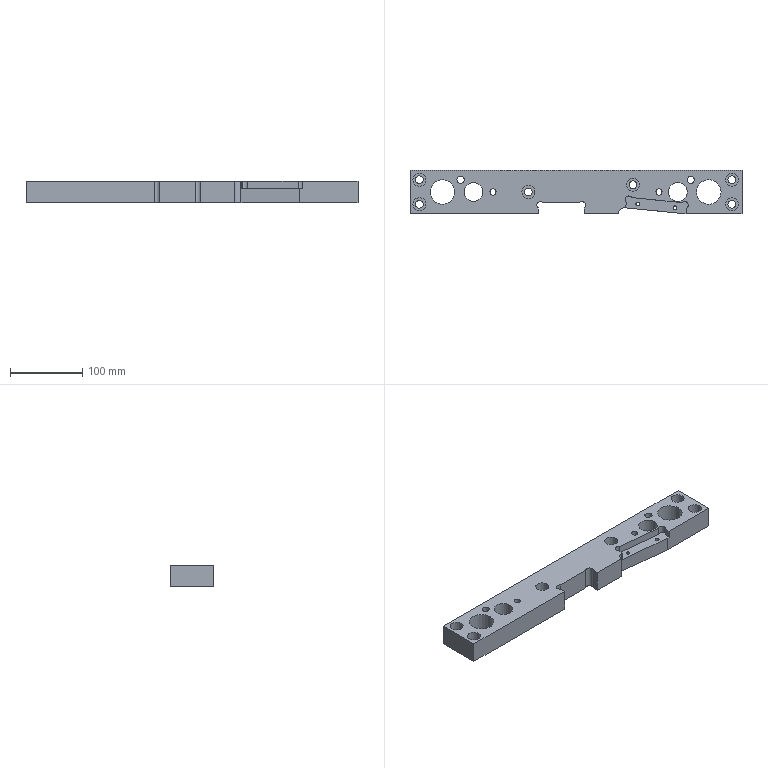Part | NX | features LIN_SOLID_COLOR 2 | 1 solid | 54 faces | box 460 x 60 x 30 mm | volume 644564 mm3 | cylinder 29 | plane 25 | commonest cylinder face diameters 11 x6 18 x6 10 x4 5.2 x2 8.5 x2 10.001 x2
STEP:
#1=CARTESIAN_POINT('',(722.839,118.195,-12.));
#2=VERTEX_POINT('',#1);
#3=CARTESIAN_POINT('',(720.239,118.195,-12.));
#4=DIRECTION('',(0.,0.,-1.));
#5=DIRECTION('',(1.,0.,0.));
#6=AXIS2_PLACEMENT_3D('',#3,#4,#5);
#7=CIRCLE('',#6,2.6);
#8=EDGE_CURVE('',#2,#2,#7,.T.);
#9=ORIENTED_EDGE('',*,*,#8,.T.);
#10=EDGE_LOOP('',(#9));
#11=FACE_BOUND('',#10,.T.);
#12=CARTESIAN_POINT('',(651.88,118.043,-12.));
#13=VERTEX_POINT('',#12);
#14=CARTESIAN_POINT('',(652.678,125.965,-12.));
#15=VERTEX_POINT('',#14);
#16=CARTESIAN_POINT('',(652.581,125.008,-12.));
#17=DIRECTION('',(0.1002,0.995,0.));
#18=VECTOR('',#17,1000.);
#19=LINE('',#16,#18);
#20=EDGE_CURVE('',#13,#15,#19,.T.);
#21=ORIENTED_EDGE('',*,*,#20,.F.);
#22=CARTESIAN_POINT('',(731.751,110.,-12.));
#23=VERTEX_POINT('',#22);
#24=CARTESIAN_POINT('',(646.905,118.544,-12.));
#25=DIRECTION('',(0.995,-0.1002,0.));
#26=VECTOR('',#25,1000.);
#27=LINE('',#24,#26);
#28=EDGE_CURVE('',#13,#23,#27,.T.);
#29=ORIENTED_EDGE('',*,*,#28,.T.);
#30=CARTESIAN_POINT('',(735.495,110.,-12.));
#31=VERTEX_POINT('',#30);
#32=CARTESIAN_POINT('',(667.,110.,-12.));
#33=DIRECTION('',(-1.,0.,0.));
#34=VECTOR('',#33,1000.);
#35=LINE('',#32,#34);
#36=EDGE_CURVE('',#31,#23,#35,.T.);
#37=ORIENTED_EDGE('',*,*,#36,.F.);
#38=CARTESIAN_POINT('',(736.255,117.548,-12.));
#39=VERTEX_POINT('',#38);
#40=CARTESIAN_POINT('',(736.159,116.592,-12.));
#41=DIRECTION('',(0.1002,0.995,0.));
#42=VECTOR('',#41,1000.);
#43=LINE('',#40,#42);
#44=EDGE_CURVE('',#31,#39,#43,.T.);
#45=ORIENTED_EDGE('',*,*,#44,.T.);
#46=CARTESIAN_POINT('',(729.957,125.257,-12.));
#47=VERTEX_POINT('',#46);
#48=CARTESIAN_POINT('',(733.475,121.704,-12.));
#49=DIRECTION('',(0.,0.,1.));
#50=DIRECTION('',(1.,0.,0.));
#51=AXIS2_PLACEMENT_3D('',#48,#49,#50);
#52=CIRCLE('',#51,5.);
#53=EDGE_CURVE('',#39,#47,#52,.T.);
#54=ORIENTED_EDGE('',*,*,#53,.T.);
#55=CARTESIAN_POINT('',(660.386,132.263,-12.));
#56=VERTEX_POINT('',#55);
#57=CARTESIAN_POINT('',(648.408,133.469,-12.));
#58=DIRECTION('',(-0.995,0.1002,0.));
#59=VECTOR('',#58,1000.);
#60=LINE('',#57,#59);
#61=EDGE_CURVE('',#56,#47,#60,.F.);
#62=ORIENTED_EDGE('',*,*,#61,.F.);
#63=CARTESIAN_POINT('',(656.23,129.483,-12.));
#64=DIRECTION('',(0.,0.,1.));
#65=DIRECTION('',(1.,0.,0.));
#66=AXIS2_PLACEMENT_3D('',#63,#64,#65);
#67=CIRCLE('',#66,5.);
#68=EDGE_CURVE('',#56,#15,#67,.T.);
#69=ORIENTED_EDGE('',*,*,#68,.T.);
#70=EDGE_LOOP('',(#21,#29,#37,#45,#54,#62,#69));
#71=FACE_BOUND('',#70,.T.);
#72=CARTESIAN_POINT('',(671.101,123.405,-12.));
#73=VERTEX_POINT('',#72);
#74=CARTESIAN_POINT('',(668.501,123.405,-12.));
#75=DIRECTION('',(0.,0.,-1.));
#76=DIRECTION('',(1.,0.,0.));
#77=AXIS2_PLACEMENT_3D('',#74,#75,#76);
#78=CIRCLE('',#77,2.6);
#79=EDGE_CURVE('',#73,#73,#78,.T.);
#80=ORIENTED_EDGE('',*,*,#79,.T.);
#81=EDGE_LOOP('',(#80));
#82=FACE_BOUND('',#81,.T.);
#83=CARTESIAN_POINT('',(647.606,125.509,-12.));
#84=DIRECTION('',(0.,0.,1.));
#85=DIRECTION('',(-0.9923,0.1236,0.));
#86=AXIS2_PLACEMENT_3D('',#83,#84,#85);
#87=PLANE('',#86);
#88=ADVANCED_FACE('',(#11,#71,#82),#87,.T.);
#89=CARTESIAN_POINT('',(693.75,140.,-1.5));
#90=VERTEX_POINT('',#89);
#91=CARTESIAN_POINT('',(698.,140.,-1.5));
#92=DIRECTION('',(0.,0.,1.));
#93=DIRECTION('',(-1.,0.,0.));
#94=AXIS2_PLACEMENT_3D('',#91,#92,#93);
#95=CIRCLE('',#94,4.25);
#96=EDGE_CURVE('',#90,#90,#95,.T.);
#97=ORIENTED_EDGE('',*,*,#96,.F.);
#98=EDGE_LOOP('',(#97));
#99=FACE_BOUND('',#98,.T.);
#100=CARTESIAN_POINT('',(472.25,140.,-1.5));
#101=VERTEX_POINT('',#100);
#102=CARTESIAN_POINT('',(468.,140.,-1.5));
#103=DIRECTION('',(0.,0.,-1.));
#104=DIRECTION('',(1.,0.,0.));
#105=AXIS2_PLACEMENT_3D('',#102,#103,#104);
#106=CIRCLE('',#105,4.25);
#107=EDGE_CURVE('',#101,#101,#106,.T.);
#108=ORIENTED_EDGE('',*,*,#107,.T.);
#109=EDGE_LOOP('',(#108));
#110=FACE_BOUND('',#109,.T.);
#111=CARTESIAN_POINT('',(671.,150.,-1.5));
#112=VERTEX_POINT('',#111);
#113=CARTESIAN_POINT('',(662.,150.,-1.5));
#114=DIRECTION('',(0.,0.,1.));
#115=DIRECTION('',(1.,0.,0.));
#116=AXIS2_PLACEMENT_3D('',#113,#114,#115);
#117=CIRCLE('',#116,9.);
#118=EDGE_CURVE('',#112,#112,#117,.T.);
#119=ORIENTED_EDGE('',*,*,#118,.F.);
#120=EDGE_LOOP('',(#119));
#121=FACE_BOUND('',#120,.T.);
#122=CARTESIAN_POINT('',(415.,140.,-1.5));
#123=VERTEX_POINT('',#122);
#124=CARTESIAN_POINT('',(398.,140.,-1.5));
#125=DIRECTION('',(0.,0.,1.));
#126=DIRECTION('',(1.,0.,0.));
#127=AXIS2_PLACEMENT_3D('',#124,#125,#126);
#128=CIRCLE('',#127,17.);
#129=EDGE_CURVE('',#123,#123,#128,.F.);
#130=ORIENTED_EDGE('',*,*,#129,.T.);
#131=EDGE_LOOP('',(#130));
#132=FACE_BOUND('',#131,.T.);
#133=CARTESIAN_POINT('',(784.,140.,-1.5));
#134=VERTEX_POINT('',#133);
#135=CARTESIAN_POINT('',(767.,140.,-1.5));
#136=DIRECTION('',(0.,0.,1.));
#137=DIRECTION('',(1.,0.,0.));
#138=AXIS2_PLACEMENT_3D('',#135,#136,#137);
#139=CIRCLE('',#138,17.);
#140=EDGE_CURVE('',#134,#134,#139,.T.);
#141=ORIENTED_EDGE('',*,*,#140,.F.);
#142=EDGE_LOOP('',(#141));
#143=FACE_BOUND('',#142,.T.);
#144=CARTESIAN_POINT('',(375.,157.,-1.5));
#145=VERTEX_POINT('',#144);
#146=CARTESIAN_POINT('',(366.,157.,-1.5));
#147=DIRECTION('',(0.,0.,1.));
#148=DIRECTION('',(1.,0.,0.));
#149=AXIS2_PLACEMENT_3D('',#146,#147,#148);
#150=CIRCLE('',#149,9.);
#151=EDGE_CURVE('',#145,#145,#150,.F.);
#152=ORIENTED_EDGE('',*,*,#151,.T.);
#153=EDGE_LOOP('',(#152));
#154=FACE_BOUND('',#153,.T.);
#155=CARTESIAN_POINT('',(375.,123.,-1.5));
#156=VERTEX_POINT('',#155);
#157=CARTESIAN_POINT('',(366.,123.,-1.5));
#158=DIRECTION('',(0.,0.,1.));
#159=DIRECTION('',(1.,0.,0.));
#160=AXIS2_PLACEMENT_3D('',#157,#158,#159);
#161=CIRCLE('',#160,9.);
#162=EDGE_CURVE('',#156,#156,#161,.F.);
#163=ORIENTED_EDGE('',*,*,#162,.T.);
#164=EDGE_LOOP('',(#163));
#165=FACE_BOUND('',#164,.T.);
#166=CARTESIAN_POINT('',(428.004,157.,-1.5));
#167=VERTEX_POINT('',#166);
#168=CARTESIAN_POINT('',(423.003,157.,-1.5));
#169=DIRECTION('',(0.,0.,1.));
#170=DIRECTION('',(1.,0.,0.));
#171=AXIS2_PLACEMENT_3D('',#168,#169,#170);
#172=CIRCLE('',#171,5.);
#173=EDGE_CURVE('',#167,#167,#172,.F.);
#174=ORIENTED_EDGE('',*,*,#173,.T.);
#175=EDGE_LOOP('',(#174));
#176=FACE_BOUND('',#175,.T.);
#177=CARTESIAN_POINT('',(526.,140.,-1.5));
#178=VERTEX_POINT('',#177);
#179=CARTESIAN_POINT('',(517.,140.,-1.5));
#180=DIRECTION('',(0.,0.,1.));
#181=DIRECTION('',(1.,0.,0.));
#182=AXIS2_PLACEMENT_3D('',#179,#180,#181);
#183=CIRCLE('',#182,9.);
#184=EDGE_CURVE('',#178,#178,#183,.F.);
#185=ORIENTED_EDGE('',*,*,#184,.T.);
#186=EDGE_LOOP('',(#185));
#187=FACE_BOUND('',#186,.T.);
#188=CARTESIAN_POINT('',(746.997,157.,-1.5));
#189=VERTEX_POINT('',#188);
#190=CARTESIAN_POINT('',(741.997,157.,-1.5));
#191=DIRECTION('',(0.,0.,1.));
#192=DIRECTION('',(1.,0.,0.));
#193=AXIS2_PLACEMENT_3D('',#190,#191,#192);
#194=CIRCLE('',#193,5.);
#195=EDGE_CURVE('',#189,#189,#194,.F.);
#196=ORIENTED_EDGE('',*,*,#195,.T.);
#197=EDGE_LOOP('',(#196));
#198=FACE_BOUND('',#197,.T.);
#199=CARTESIAN_POINT('',(808.,157.,-1.5));
#200=VERTEX_POINT('',#199);
#201=CARTESIAN_POINT('',(799.,157.,-1.5));
#202=DIRECTION('',(0.,0.,1.));
#203=DIRECTION('',(1.,0.,0.));
#204=AXIS2_PLACEMENT_3D('',#201,#202,#203);
#205=CIRCLE('',#204,9.);
#206=EDGE_CURVE('',#200,#200,#205,.F.);
#207=ORIENTED_EDGE('',*,*,#206,.T.);
#208=EDGE_LOOP('',(#207));
#209=FACE_BOUND('',#208,.T.);
#210=CARTESIAN_POINT('',(808.,123.,-1.5));
#211=VERTEX_POINT('',#210);
#212=CARTESIAN_POINT('',(799.,123.,-1.5));
#213=DIRECTION('',(0.,0.,1.));
#214=DIRECTION('',(1.,0.,0.));
#215=AXIS2_PLACEMENT_3D('',#212,#213,#214);
#216=CIRCLE('',#215,9.);
#217=EDGE_CURVE('',#211,#211,#216,.F.);
#218=ORIENTED_EDGE('',*,*,#217,.T.);
#219=EDGE_LOOP('',(#218));
#220=FACE_BOUND('',#219,.T.);
#221=CARTESIAN_POINT('',(737.,140.,-1.5));
#222=VERTEX_POINT('',#221);
#223=CARTESIAN_POINT('',(724.,140.,-1.5));
#224=DIRECTION('',(0.,0.,-1.));
#225=DIRECTION('',(1.,0.,0.));
#226=AXIS2_PLACEMENT_3D('',#223,#224,#225);
#227=CIRCLE('',#226,13.);
#228=EDGE_CURVE('',#222,#222,#227,.T.);
#229=ORIENTED_EDGE('',*,*,#228,.T.);
#230=EDGE_LOOP('',(#229));
#231=FACE_BOUND('',#230,.T.);
#232=CARTESIAN_POINT('',(454.,140.,-1.5));
#233=VERTEX_POINT('',#232);
#234=CARTESIAN_POINT('',(441.,140.,-1.5));
#235=DIRECTION('',(0.,0.,-1.));
#236=DIRECTION('',(1.,0.,0.));
#237=AXIS2_PLACEMENT_3D('',#234,#235,#236);
#238=CIRCLE('',#237,13.);
#239=EDGE_CURVE('',#233,#233,#238,.F.);
#240=ORIENTED_EDGE('',*,*,#239,.F.);
#241=EDGE_LOOP('',(#240));
#242=FACE_BOUND('',#241,.T.);
#243=CARTESIAN_POINT('',(530.5,110.,-1.5));
#244=VERTEX_POINT('',#243);
#245=CARTESIAN_POINT('',(530.5,117.961,-1.5));
#246=VERTEX_POINT('',#245);
#247=CARTESIAN_POINT('',(530.5,0.,-1.5));
#248=DIRECTION('',(0.,1.,0.));
#249=VECTOR('',#248,1000.);
#250=LINE('',#247,#249);
#251=EDGE_CURVE('',#244,#246,#250,.T.);
#252=ORIENTED_EDGE('',*,*,#251,.T.);
#253=CARTESIAN_POINT('',(537.539,125.,-1.5));
#254=VERTEX_POINT('',#253);
#255=CARTESIAN_POINT('',(533.682,121.818,-1.5));
#256=DIRECTION('',(0.,0.,-1.));
#257=DIRECTION('',(1.,0.,0.));
#258=AXIS2_PLACEMENT_3D('',#255,#256,#257);
#259=CIRCLE('',#258,5.);
#260=EDGE_CURVE('',#246,#254,#259,.T.);
#261=ORIENTED_EDGE('',*,*,#260,.T.);
#262=CARTESIAN_POINT('',(587.461,125.,-1.5));
#263=VERTEX_POINT('',#262);
#264=CARTESIAN_POINT('',(630.2,125.,-1.5));
#265=DIRECTION('',(-1.,0.,0.));
#266=VECTOR('',#265,1000.);
#267=LINE('',#264,#266);
#268=EDGE_CURVE('',#263,#254,#267,.T.);
#269=ORIENTED_EDGE('',*,*,#268,.F.);
#270=CARTESIAN_POINT('',(594.5,117.961,-1.5));
#271=VERTEX_POINT('',#270);
#272=CARTESIAN_POINT('',(591.318,121.818,-1.5));
#273=DIRECTION('',(0.,0.,-1.));
#274=DIRECTION('',(1.,0.,0.));
#275=AXIS2_PLACEMENT_3D('',#272,#273,#274);
#276=CIRCLE('',#275,5.);
#277=EDGE_CURVE('',#263,#271,#276,.T.);
#278=ORIENTED_EDGE('',*,*,#277,.T.);
#279=CARTESIAN_POINT('',(594.5,110.,-1.5));
#280=VERTEX_POINT('',#279);
#281=CARTESIAN_POINT('',(594.5,173.255,-1.5));
#282=DIRECTION('',(0.,-1.,0.));
#283=VECTOR('',#282,1000.);
#284=LINE('',#281,#283);
#285=EDGE_CURVE('',#271,#280,#284,.T.);
#286=ORIENTED_EDGE('',*,*,#285,.T.);
#287=CARTESIAN_POINT('',(642.024,110.,-1.5));
#288=VERTEX_POINT('',#287);
#289=CARTESIAN_POINT('',(667.,110.,-1.5));
#290=DIRECTION('',(-1.,0.,0.));
#291=VECTOR('',#290,1000.);
#292=LINE('',#289,#291);
#293=EDGE_CURVE('',#280,#288,#292,.F.);
#294=ORIENTED_EDGE('',*,*,#293,.T.);
#295=CARTESIAN_POINT('',(642.124,110.985,-1.5));
#296=VERTEX_POINT('',#295);
#297=CARTESIAN_POINT('',(648.212,171.442,-1.5));
#298=DIRECTION('',(-0.1002,-0.995,0.));
#299=VECTOR('',#298,1000.);
#300=LINE('',#297,#299);
#301=EDGE_CURVE('',#296,#288,#300,.T.);
#302=ORIENTED_EDGE('',*,*,#301,.F.);
#303=CARTESIAN_POINT('',(650.885,118.144,-1.5));
#304=VERTEX_POINT('',#303);
#305=CARTESIAN_POINT('',(650.083,110.184,-1.5));
#306=DIRECTION('',(0.,0.,1.));
#307=DIRECTION('',(1.,0.,0.));
#308=AXIS2_PLACEMENT_3D('',#305,#306,#307);
#309=CIRCLE('',#308,8.);
#310=EDGE_CURVE('',#304,#296,#309,.T.);
#311=ORIENTED_EDGE('',*,*,#310,.F.);
#312=CARTESIAN_POINT('',(651.88,118.043,-1.5));
#313=VERTEX_POINT('',#312);
#314=CARTESIAN_POINT('',(624.913,120.759,-1.5));
#315=DIRECTION('',(0.995,-0.1002,0.));
#316=VECTOR('',#315,1000.);
#317=LINE('',#314,#316);
#318=EDGE_CURVE('',#304,#313,#317,.T.);
#319=ORIENTED_EDGE('',*,*,#318,.T.);
#320=CARTESIAN_POINT('',(652.678,125.965,-1.5));
#321=VERTEX_POINT('',#320);
#322=CARTESIAN_POINT('',(657.167,170.54,-1.5));
#323=DIRECTION('',(0.1002,0.995,0.));
#324=VECTOR('',#323,1000.);
#325=LINE('',#322,#324);
#326=EDGE_CURVE('',#313,#321,#325,.T.);
#327=ORIENTED_EDGE('',*,*,#326,.T.);
#328=CARTESIAN_POINT('',(660.386,132.263,-1.5));
#329=VERTEX_POINT('',#328);
#330=CARTESIAN_POINT('',(656.23,129.483,-1.5));
#331=DIRECTION('',(0.,0.,1.));
#332=DIRECTION('',(1.,0.,0.));
#333=AXIS2_PLACEMENT_3D('',#330,#331,#332);
#334=CIRCLE('',#333,5.);
#335=EDGE_CURVE('',#329,#321,#334,.T.);
#336=ORIENTED_EDGE('',*,*,#335,.F.);
#337=CARTESIAN_POINT('',(729.957,125.257,-1.5));
#338=VERTEX_POINT('',#337);
#339=CARTESIAN_POINT('',(626.416,135.684,-1.5));
#340=DIRECTION('',(-0.995,0.1002,0.));
#341=VECTOR('',#340,1000.);
#342=LINE('',#339,#341);
#343=EDGE_CURVE('',#338,#329,#342,.T.);
#344=ORIENTED_EDGE('',*,*,#343,.F.);
#345=CARTESIAN_POINT('',(736.255,117.548,-1.5));
#346=VERTEX_POINT('',#345);
#347=CARTESIAN_POINT('',(733.475,121.704,-1.5));
#348=DIRECTION('',(0.,0.,1.));
#349=DIRECTION('',(1.,0.,0.));
#350=AXIS2_PLACEMENT_3D('',#347,#348,#349);
#351=CIRCLE('',#350,5.);
#352=EDGE_CURVE('',#346,#338,#351,.T.);
#353=ORIENTED_EDGE('',*,*,#352,.F.);
#354=CARTESIAN_POINT('',(735.495,110.,-1.5));
#355=VERTEX_POINT('',#354);
#356=CARTESIAN_POINT('',(740.744,162.123,-1.5));
#357=DIRECTION('',(-0.1002,-0.995,0.));
#358=VECTOR('',#357,1000.);
#359=LINE('',#356,#358);
#360=EDGE_CURVE('',#346,#355,#359,.T.);
#361=ORIENTED_EDGE('',*,*,#360,.T.);
#362=CARTESIAN_POINT('',(813.,110.,-1.5));
#363=VERTEX_POINT('',#362);
#364=CARTESIAN_POINT('',(667.,110.,-1.5));
#365=DIRECTION('',(-1.,0.,0.));
#366=VECTOR('',#365,1000.);
#367=LINE('',#364,#366);
#368=EDGE_CURVE('',#355,#363,#367,.F.);
#369=ORIENTED_EDGE('',*,*,#368,.T.);
#370=CARTESIAN_POINT('',(813.,170.,-1.5));
#371=VERTEX_POINT('',#370);
#372=CARTESIAN_POINT('',(813.,30.,-1.5));
#373=DIRECTION('',(0.,-1.,0.));
#374=VECTOR('',#373,1000.);
#375=LINE('',#372,#374);
#376=EDGE_CURVE('',#371,#363,#375,.T.);
#377=ORIENTED_EDGE('',*,*,#376,.F.);
#378=CARTESIAN_POINT('',(353.,170.,-1.5));
#379=VERTEX_POINT('',#378);
#380=CARTESIAN_POINT('',(667.,170.,-1.5));
#381=DIRECTION('',(1.,0.,0.));
#382=VECTOR('',#381,1000.);
#383=LINE('',#380,#382);
#384=EDGE_CURVE('',#371,#379,#383,.F.);
#385=ORIENTED_EDGE('',*,*,#384,.T.);
#386=CARTESIAN_POINT('',(353.,110.,-1.5));
#387=VERTEX_POINT('',#386);
#388=CARTESIAN_POINT('',(353.,30.,-1.5));
#389=DIRECTION('',(0.,-1.,0.));
#390=VECTOR('',#389,1000.);
#391=LINE('',#388,#390);
#392=EDGE_CURVE('',#379,#387,#391,.T.);
#393=ORIENTED_EDGE('',*,*,#392,.T.);
#394=CARTESIAN_POINT('',(667.,110.,-1.5));
#395=DIRECTION('',(-1.,0.,0.));
#396=VECTOR('',#395,1000.);
#397=LINE('',#394,#396);
#398=EDGE_CURVE('',#387,#244,#397,.F.);
#399=ORIENTED_EDGE('',*,*,#398,.T.);
#400=EDGE_LOOP('',(#252,#261,#269,#278,#286,#294,#302,#311,#319,#327,#336,#344,#353,#361,#369,#377,#385,#393,#399));
#401=FACE_BOUND('',#400,.T.);
#402=CARTESIAN_POINT('',(630.2,173.255,-1.5));
#403=DIRECTION('',(0.,0.,1.));
#404=DIRECTION('',(1.,0.,0.));
#405=AXIS2_PLACEMENT_3D('',#402,#403,#404);
#406=PLANE('',#405);
#407=ADVANCED_FACE('',(#99,#110,#121,#132,#143,#154,#165,#176,#187,#198,#209,#220,#231,#242,#401),#406,.T.);
#408=CARTESIAN_POINT('',(665.901,123.405,-31.5));
#409=VERTEX_POINT('',#408);
#410=CARTESIAN_POINT('',(668.501,123.405,-31.5));
#411=DIRECTION('',(0.,0.,-1.));
#412=DIRECTION('',(-1.,0.,0.));
#413=AXIS2_PLACEMENT_3D('',#410,#411,#412);
#414=CIRCLE('',#413,2.6);
#415=EDGE_CURVE('',#409,#409,#414,.T.);
#416=ORIENTED_EDGE('',*,*,#415,.F.);
#417=EDGE_LOOP('',(#416));
#418=FACE_BOUND('',#417,.T.);
#419=CARTESIAN_POINT('',(717.639,118.195,-31.5));
#420=VERTEX_POINT('',#419);
#421=CARTESIAN_POINT('',(720.239,118.195,-31.5));
#422=DIRECTION('',(0.,0.,-1.));
#423=DIRECTION('',(-1.,0.,0.));
#424=AXIS2_PLACEMENT_3D('',#421,#422,#423);
#425=CIRCLE('',#424,2.6);
#426=EDGE_CURVE('',#420,#420,#425,.T.);
#427=ORIENTED_EDGE('',*,*,#426,.F.);
#428=EDGE_LOOP('',(#427));
#429=FACE_BOUND('',#428,.T.);
#430=CARTESIAN_POINT('',(463.75,140.,-31.5));
#431=VERTEX_POINT('',#430);
#432=CARTESIAN_POINT('',(468.,140.,-31.5));
#433=DIRECTION('',(0.,0.,-1.));
#434=DIRECTION('',(-1.,0.,0.));
#435=AXIS2_PLACEMENT_3D('',#432,#433,#434);
#436=CIRCLE('',#435,4.25);
#437=EDGE_CURVE('',#431,#431,#436,.T.);
#438=ORIENTED_EDGE('',*,*,#437,.F.);
#439=EDGE_LOOP('',(#438));
#440=FACE_BOUND('',#439,.T.);
#441=CARTESIAN_POINT('',(693.75,140.,-31.5));
#442=VERTEX_POINT('',#441);
#443=CARTESIAN_POINT('',(698.,140.,-31.5));
#444=DIRECTION('',(0.,0.,-1.));
#445=DIRECTION('',(-1.,0.,0.));
#446=AXIS2_PLACEMENT_3D('',#443,#444,#445);
#447=CIRCLE('',#446,4.25);
#448=EDGE_CURVE('',#442,#442,#447,.T.);
#449=ORIENTED_EDGE('',*,*,#448,.F.);
#450=EDGE_LOOP('',(#449));
#451=FACE_BOUND('',#450,.T.);
#452=CARTESIAN_POINT('',(428.,140.,-31.5));
#453=VERTEX_POINT('',#452);
#454=CARTESIAN_POINT('',(441.,140.,-31.5));
#455=DIRECTION('',(0.,0.,1.));
#456=DIRECTION('',(-1.,0.,0.));
#457=AXIS2_PLACEMENT_3D('',#454,#455,#456);
#458=CIRCLE('',#457,13.);
#459=EDGE_CURVE('',#453,#453,#458,.F.);
#460=ORIENTED_EDGE('',*,*,#459,.F.);
#461=EDGE_LOOP('',(#460));
#462=FACE_BOUND('',#461,.T.);
#463=CARTESIAN_POINT('',(711.,140.,-31.5));
#464=VERTEX_POINT('',#463);
#465=CARTESIAN_POINT('',(724.,140.,-31.5));
#466=DIRECTION('',(0.,0.,1.));
#467=DIRECTION('',(-1.,0.,0.));
#468=AXIS2_PLACEMENT_3D('',#465,#466,#467);
#469=CIRCLE('',#468,13.);
#470=EDGE_CURVE('',#464,#464,#469,.T.);
#471=ORIENTED_EDGE('',*,*,#470,.T.);
#472=EDGE_LOOP('',(#471));
#473=FACE_BOUND('',#472,.T.);
#474=CARTESIAN_POINT('',(793.5,123.,-31.5));
#475=VERTEX_POINT('',#474);
#476=CARTESIAN_POINT('',(799.,123.,-31.5));
#477=DIRECTION('',(0.,0.,-1.));
#478=DIRECTION('',(-1.,0.,0.));
#479=AXIS2_PLACEMENT_3D('',#476,#477,#478);
#480=CIRCLE('',#479,5.5);
#481=EDGE_CURVE('',#475,#475,#480,.F.);
#482=ORIENTED_EDGE('',*,*,#481,.T.);
#483=EDGE_LOOP('',(#482));
#484=FACE_BOUND('',#483,.T.);
#485=CARTESIAN_POINT('',(793.5,157.,-31.5));
#486=VERTEX_POINT('',#485);
#487=CARTESIAN_POINT('',(799.,157.,-31.5));
#488=DIRECTION('',(0.,0.,-1.));
#489=DIRECTION('',(-1.,0.,0.));
#490=AXIS2_PLACEMENT_3D('',#487,#488,#489);
#491=CIRCLE('',#490,5.5);
#492=EDGE_CURVE('',#486,#486,#491,.F.);
#493=ORIENTED_EDGE('',*,*,#492,.T.);
#494=EDGE_LOOP('',(#493));
#495=FACE_BOUND('',#494,.T.);
#496=CARTESIAN_POINT('',(736.996,157.,-31.5));
#497=VERTEX_POINT('',#496);
#498=CARTESIAN_POINT('',(741.997,157.,-31.5));
#499=DIRECTION('',(0.,0.,-1.));
#500=DIRECTION('',(-1.,0.,0.));
#501=AXIS2_PLACEMENT_3D('',#498,#499,#500);
#502=CIRCLE('',#501,5.);
#503=EDGE_CURVE('',#497,#497,#502,.F.);
#504=ORIENTED_EDGE('',*,*,#503,.T.);
#505=EDGE_LOOP('',(#504));
#506=FACE_BOUND('',#505,.T.);
#507=CARTESIAN_POINT('',(511.5,140.,-31.5));
#508=VERTEX_POINT('',#507);
#509=CARTESIAN_POINT('',(517.,140.,-31.5));
#510=DIRECTION('',(0.,0.,-1.));
#511=DIRECTION('',(-1.,0.,0.));
#512=AXIS2_PLACEMENT_3D('',#509,#510,#511);
#513=CIRCLE('',#512,5.5);
#514=EDGE_CURVE('',#508,#508,#513,.F.);
#515=ORIENTED_EDGE('',*,*,#514,.T.);
#516=EDGE_LOOP('',(#515));
#517=FACE_BOUND('',#516,.T.);
#518=CARTESIAN_POINT('',(379.,140.,-31.5));
#519=VERTEX_POINT('',#518);
#520=CARTESIAN_POINT('',(398.,140.,-31.5));
#521=DIRECTION('',(0.,0.,-1.));
#522=DIRECTION('',(-1.,0.,0.));
#523=AXIS2_PLACEMENT_3D('',#520,#521,#522);
#524=CIRCLE('',#523,19.);
#525=EDGE_CURVE('',#519,#519,#524,.T.);
#526=ORIENTED_EDGE('',*,*,#525,.F.);
#527=EDGE_LOOP('',(#526));
#528=FACE_BOUND('',#527,.T.);
#529=CARTESIAN_POINT('',(748.,140.,-31.5));
#530=VERTEX_POINT('',#529);
#531=CARTESIAN_POINT('',(767.,140.,-31.5));
#532=DIRECTION('',(0.,0.,-1.));
#533=DIRECTION('',(-1.,0.,0.));
#534=AXIS2_PLACEMENT_3D('',#531,#532,#533);
#535=CIRCLE('',#534,19.);
#536=EDGE_CURVE('',#530,#530,#535,.F.);
#537=ORIENTED_EDGE('',*,*,#536,.T.);
#538=EDGE_LOOP('',(#537));
#539=FACE_BOUND('',#538,.T.);
#540=CARTESIAN_POINT('',(360.5,157.,-31.5));
#541=VERTEX_POINT('',#540);
#542=CARTESIAN_POINT('',(366.,157.,-31.5));
#543=DIRECTION('',(0.,0.,-1.));
#544=DIRECTION('',(-1.,0.,0.));
#545=AXIS2_PLACEMENT_3D('',#542,#543,#544);
#546=CIRCLE('',#545,5.5);
#547=EDGE_CURVE('',#541,#541,#546,.F.);
#548=ORIENTED_EDGE('',*,*,#547,.T.);
#549=EDGE_LOOP('',(#548));
#550=FACE_BOUND('',#549,.T.);
#551=CARTESIAN_POINT('',(360.5,123.,-31.5));
#552=VERTEX_POINT('',#551);
#553=CARTESIAN_POINT('',(366.,123.,-31.5));
#554=DIRECTION('',(0.,0.,-1.));
#555=DIRECTION('',(-1.,0.,0.));
#556=AXIS2_PLACEMENT_3D('',#553,#554,#555);
#557=CIRCLE('',#556,5.5);
#558=EDGE_CURVE('',#552,#552,#557,.F.);
#559=ORIENTED_EDGE('',*,*,#558,.T.);
#560=EDGE_LOOP('',(#559));
#561=FACE_BOUND('',#560,.T.);
#562=CARTESIAN_POINT('',(418.003,157.,-31.5));
#563=VERTEX_POINT('',#562);
#564=CARTESIAN_POINT('',(423.003,157.,-31.5));
#565=DIRECTION('',(0.,0.,-1.));
#566=DIRECTION('',(-1.,0.,0.));
#567=AXIS2_PLACEMENT_3D('',#564,#565,#566);
#568=CIRCLE('',#567,5.);
#569=EDGE_CURVE('',#563,#563,#568,.T.);
#570=ORIENTED_EDGE('',*,*,#569,.F.);
#571=EDGE_LOOP('',(#570));
#572=FACE_BOUND('',#571,.T.);
#573=CARTESIAN_POINT('',(656.5,150.,-31.5));
#574=VERTEX_POINT('',#573);
#575=CARTESIAN_POINT('',(662.,150.,-31.5));
#576=DIRECTION('',(0.,0.,-1.));
#577=DIRECTION('',(-1.,0.,0.));
#578=AXIS2_PLACEMENT_3D('',#575,#576,#577);
#579=CIRCLE('',#578,5.5);
#580=EDGE_CURVE('',#574,#574,#579,.T.);
#581=ORIENTED_EDGE('',*,*,#580,.F.);
#582=EDGE_LOOP('',(#581));
#583=FACE_BOUND('',#582,.T.);
#584=CARTESIAN_POINT('',(537.539,125.,-31.5));
#585=VERTEX_POINT('',#584);
#586=CARTESIAN_POINT('',(587.461,125.,-31.5));
#587=VERTEX_POINT('',#586);
#588=CARTESIAN_POINT('',(667.,125.,-31.5));
#589=DIRECTION('',(1.,0.,0.));
#590=VECTOR('',#589,1000.);
#591=LINE('',#588,#590);
#592=EDGE_CURVE('',#585,#587,#591,.T.);
#593=ORIENTED_EDGE('',*,*,#592,.F.);
#594=CARTESIAN_POINT('',(530.5,117.961,-31.5));
#595=VERTEX_POINT('',#594);
#596=CARTESIAN_POINT('',(533.682,121.818,-31.5));
#597=DIRECTION('',(0.,0.,1.));
#598=DIRECTION('',(1.,0.,0.));
#599=AXIS2_PLACEMENT_3D('',#596,#597,#598);
#600=CIRCLE('',#599,5.);
#601=EDGE_CURVE('',#585,#595,#600,.T.);
#602=ORIENTED_EDGE('',*,*,#601,.T.);
#603=CARTESIAN_POINT('',(530.5,110.,-31.5));
#604=VERTEX_POINT('',#603);
#605=CARTESIAN_POINT('',(530.5,0.,-31.5));
#606=DIRECTION('',(0.,-1.,0.));
#607=VECTOR('',#606,1000.);
#608=LINE('',#605,#607);
#609=EDGE_CURVE('',#595,#604,#608,.T.);
#610=ORIENTED_EDGE('',*,*,#609,.T.);
#611=CARTESIAN_POINT('',(353.,110.,-31.5));
#612=VERTEX_POINT('',#611);
#613=CARTESIAN_POINT('',(667.,110.,-31.5));
#614=DIRECTION('',(1.,0.,0.));
#615=VECTOR('',#614,1000.);
#616=LINE('',#613,#615);
#617=EDGE_CURVE('',#604,#612,#616,.F.);
#618=ORIENTED_EDGE('',*,*,#617,.T.);
#619=CARTESIAN_POINT('',(353.,170.,-31.5));
#620=VERTEX_POINT('',#619);
#621=CARTESIAN_POINT('',(353.,30.,-31.5));
#622=DIRECTION('',(0.,1.,0.));
#623=VECTOR('',#622,1000.);
#624=LINE('',#621,#623);
#625=EDGE_CURVE('',#612,#620,#624,.T.);
#626=ORIENTED_EDGE('',*,*,#625,.T.);
#627=CARTESIAN_POINT('',(813.,170.,-31.5));
#628=VERTEX_POINT('',#627);
#629=CARTESIAN_POINT('',(667.,170.,-31.5));
#630=DIRECTION('',(-1.,0.,0.));
#631=VECTOR('',#630,1000.);
#632=LINE('',#629,#631);
#633=EDGE_CURVE('',#620,#628,#632,.F.);
#634=ORIENTED_EDGE('',*,*,#633,.T.);
#635=CARTESIAN_POINT('',(813.,110.,-31.5));
#636=VERTEX_POINT('',#635);
#637=CARTESIAN_POINT('',(813.,30.,-31.5));
#638=DIRECTION('',(0.,1.,0.));
#639=VECTOR('',#638,1000.);
#640=LINE('',#637,#639);
#641=EDGE_CURVE('',#636,#628,#640,.T.);
#642=ORIENTED_EDGE('',*,*,#641,.F.);
#643=CARTESIAN_POINT('',(731.751,110.,-31.5));
#644=VERTEX_POINT('',#643);
#645=CARTESIAN_POINT('',(667.,110.,-31.5));
#646=DIRECTION('',(1.,0.,0.));
#647=VECTOR('',#646,1000.);
#648=LINE('',#645,#647);
#649=EDGE_CURVE('',#636,#644,#648,.F.);
#650=ORIENTED_EDGE('',*,*,#649,.T.);
#651=CARTESIAN_POINT('',(650.885,118.144,-31.5));
#652=VERTEX_POINT('',#651);
#653=CARTESIAN_POINT('',(652.875,117.943,-31.5));
#654=DIRECTION('',(0.995,-0.1002,0.));
#655=VECTOR('',#654,1000.);
#656=LINE('',#653,#655);
#657=EDGE_CURVE('',#652,#644,#656,.T.);
#658=ORIENTED_EDGE('',*,*,#657,.F.);
#659=CARTESIAN_POINT('',(642.124,110.985,-31.5));
#660=VERTEX_POINT('',#659);
#661=CARTESIAN_POINT('',(650.083,110.184,-31.5));
#662=DIRECTION('',(0.,0.,-1.));
#663=DIRECTION('',(-1.,0.,0.));
#664=AXIS2_PLACEMENT_3D('',#661,#662,#663);
#665=CIRCLE('',#664,8.);
#666=EDGE_CURVE('',#660,#652,#665,.T.);
#667=ORIENTED_EDGE('',*,*,#666,.F.);
#668=CARTESIAN_POINT('',(642.024,110.,-31.5));
#669=VERTEX_POINT('',#668);
#670=CARTESIAN_POINT('',(645.266,142.189,-31.5));
#671=DIRECTION('',(0.1002,0.995,0.));
#672=VECTOR('',#671,1000.);
#673=LINE('',#670,#672);
#674=EDGE_CURVE('',#669,#660,#673,.T.);
#675=ORIENTED_EDGE('',*,*,#674,.F.);
#676=CARTESIAN_POINT('',(594.5,110.,-31.5));
#677=VERTEX_POINT('',#676);
#678=CARTESIAN_POINT('',(667.,110.,-31.5));
#679=DIRECTION('',(1.,0.,0.));
#680=VECTOR('',#679,1000.);
#681=LINE('',#678,#680);
#682=EDGE_CURVE('',#669,#677,#681,.F.);
#683=ORIENTED_EDGE('',*,*,#682,.T.);
#684=CARTESIAN_POINT('',(594.5,117.961,-31.5));
#685=VERTEX_POINT('',#684);
#686=CARTESIAN_POINT('',(594.5,140.,-31.5));
#687=DIRECTION('',(0.,1.,0.));
#688=VECTOR('',#687,1000.);
#689=LINE('',#686,#688);
#690=EDGE_CURVE('',#677,#685,#689,.T.);
#691=ORIENTED_EDGE('',*,*,#690,.T.);
#692=CARTESIAN_POINT('',(591.318,121.818,-31.5));
#693=DIRECTION('',(0.,0.,1.));
#694=DIRECTION('',(1.,0.,0.));
#695=AXIS2_PLACEMENT_3D('',#692,#693,#694);
#696=CIRCLE('',#695,5.);
#697=EDGE_CURVE('',#685,#587,#696,.T.);
#698=ORIENTED_EDGE('',*,*,#697,.T.);
#699=EDGE_LOOP('',(#593,#602,#610,#618,#626,#634,#642,#650,#658,#667,#675,#683,#691,#698));
#700=FACE_BOUND('',#699,.T.);
#701=CARTESIAN_POINT('',(667.,140.,-31.5));
#702=DIRECTION('',(0.,0.,-1.));
#703=DIRECTION('',(1.,0.,0.));
#704=AXIS2_PLACEMENT_3D('',#701,#702,#703);
#705=PLANE('',#704);
#706=ADVANCED_FACE('',(#418,#429,#440,#451,#462,#473,#484,#495,#506,#517,#528,#539,#550,#561,#572,#583,#700),#705,.T.);
#707=ORIENTED_EDGE('',*,*,#293,.F.);
#708=CARTESIAN_POINT('',(594.5,110.,-41.5));
#709=DIRECTION('',(0.,0.,-1.));
#710=VECTOR('',#709,1000.);
#711=LINE('',#708,#710);
#712=EDGE_CURVE('',#280,#677,#711,.T.);
#713=ORIENTED_EDGE('',*,*,#712,.T.);
#714=ORIENTED_EDGE('',*,*,#682,.F.);
#715=CARTESIAN_POINT('',(642.024,110.,-41.5));
#716=DIRECTION('',(0.,0.,-1.));
#717=VECTOR('',#716,1000.);
#718=LINE('',#715,#717);
#719=EDGE_CURVE('',#288,#669,#718,.T.);
#720=ORIENTED_EDGE('',*,*,#719,.F.);
#721=EDGE_LOOP('',(#707,#713,#714,#720));
#722=FACE_BOUND('',#721,.T.);
#723=CARTESIAN_POINT('',(667.,110.,-41.5));
#724=DIRECTION('',(0.,-1.,0.));
#725=DIRECTION('',(0.,0.,1.));
#726=AXIS2_PLACEMENT_3D('',#723,#724,#725);
#727=PLANE('',#726);
#728=ADVANCED_FACE('',(#722),#727,.T.);
#729=CARTESIAN_POINT('',(731.751,110.,-41.5));
#730=DIRECTION('',(0.,0.,-1.));
#731=VECTOR('',#730,1000.);
#732=LINE('',#729,#731);
#733=EDGE_CURVE('',#23,#644,#732,.T.);
#734=ORIENTED_EDGE('',*,*,#733,.T.);
#735=ORIENTED_EDGE('',*,*,#649,.F.);
#736=CARTESIAN_POINT('',(813.,110.,-41.5));
#737=DIRECTION('',(0.,0.,1.));
#738=VECTOR('',#737,1000.);
#739=LINE('',#736,#738);
#740=EDGE_CURVE('',#636,#363,#739,.T.);
#741=ORIENTED_EDGE('',*,*,#740,.T.);
#742=ORIENTED_EDGE('',*,*,#368,.F.);
#743=CARTESIAN_POINT('',(735.495,110.,-41.5));
#744=DIRECTION('',(0.,0.,-1.));
#745=VECTOR('',#744,1000.);
#746=LINE('',#743,#745);
#747=EDGE_CURVE('',#355,#31,#746,.T.);
#748=ORIENTED_EDGE('',*,*,#747,.T.);
#749=ORIENTED_EDGE('',*,*,#36,.T.);
#750=EDGE_LOOP('',(#734,#735,#741,#742,#748,#749));
#751=FACE_BOUND('',#750,.T.);
#752=CARTESIAN_POINT('',(667.,110.,-41.5));
#753=DIRECTION('',(0.,-1.,0.));
#754=DIRECTION('',(0.,0.,1.));
#755=AXIS2_PLACEMENT_3D('',#752,#753,#754);
#756=PLANE('',#755);
#757=ADVANCED_FACE('',(#751),#756,.T.);
#758=ORIENTED_EDGE('',*,*,#326,.F.);
#759=CARTESIAN_POINT('',(651.88,118.043,50.));
#760=DIRECTION('',(0.,0.,-1.));
#761=VECTOR('',#760,1000.);
#762=LINE('',#759,#761);
#763=EDGE_CURVE('',#313,#13,#762,.T.);
#764=ORIENTED_EDGE('',*,*,#763,.T.);
#765=ORIENTED_EDGE('',*,*,#20,.T.);
#766=CARTESIAN_POINT('',(652.678,125.965,-12.));
#767=DIRECTION('',(0.,0.,1.));
#768=VECTOR('',#767,1000.);
#769=LINE('',#766,#768);
#770=EDGE_CURVE('',#321,#15,#769,.F.);
#771=ORIENTED_EDGE('',*,*,#770,.F.);
#772=EDGE_LOOP('',(#758,#764,#765,#771));
#773=FACE_BOUND('',#772,.T.);
#774=CARTESIAN_POINT('',(652.581,125.008,50.));
#775=DIRECTION('',(0.995,-0.1002,0.));
#776=DIRECTION('',(0.1002,0.995,0.));
#777=AXIS2_PLACEMENT_3D('',#774,#775,#776);
#778=PLANE('',#777);
#779=ADVANCED_FACE('',(#773),#778,.T.);
#780=CARTESIAN_POINT('',(530.5,110.,-41.5));
#781=DIRECTION('',(0.,0.,-1.));
#782=VECTOR('',#781,1000.);
#783=LINE('',#780,#782);
#784=EDGE_CURVE('',#244,#604,#783,.T.);
#785=ORIENTED_EDGE('',*,*,#784,.F.);
#786=ORIENTED_EDGE('',*,*,#398,.F.);
#787=CARTESIAN_POINT('',(353.,110.,-41.5));
#788=DIRECTION('',(0.,0.,1.));
#789=VECTOR('',#788,1000.);
#790=LINE('',#787,#789);
#791=EDGE_CURVE('',#612,#387,#790,.T.);
#792=ORIENTED_EDGE('',*,*,#791,.F.);
#793=ORIENTED_EDGE('',*,*,#617,.F.);
#794=EDGE_LOOP('',(#785,#786,#792,#793));
#795=FACE_BOUND('',#794,.T.);
#796=CARTESIAN_POINT('',(667.,110.,-41.5));
#797=DIRECTION('',(0.,-1.,0.));
#798=DIRECTION('',(0.,0.,1.));
#799=AXIS2_PLACEMENT_3D('',#796,#797,#798);
#800=PLANE('',#799);
#801=ADVANCED_FACE('',(#795),#800,.T.);
#802=ORIENTED_EDGE('',*,*,#118,.T.);
#803=EDGE_LOOP('',(#802));
#804=FACE_BOUND('',#803,.T.);
#805=CARTESIAN_POINT('',(653.,150.,-16.5));
#806=VERTEX_POINT('',#805);
#807=CARTESIAN_POINT('',(662.,150.,-16.5));
#808=DIRECTION('',(0.,0.,-1.));
#809=DIRECTION('',(-1.,0.,0.));
#810=AXIS2_PLACEMENT_3D('',#807,#808,#809);
#811=CIRCLE('',#810,9.);
#812=EDGE_CURVE('',#806,#806,#811,.T.);
#813=ORIENTED_EDGE('',*,*,#812,.T.);
#814=EDGE_LOOP('',(#813));
#815=FACE_BOUND('',#814,.T.);
#816=CARTESIAN_POINT('',(662.,150.,-16.5));
#817=DIRECTION('',(0.,0.,1.));
#818=DIRECTION('',(1.,0.,0.));
#819=AXIS2_PLACEMENT_3D('',#816,#817,#818);
#820=CYLINDRICAL_SURFACE('',#819,9.);
#821=ADVANCED_FACE('',(#804,#815),#820,.F.);
#822=ORIENTED_EDGE('',*,*,#812,.F.);
#823=EDGE_LOOP('',(#822));
#824=FACE_BOUND('',#823,.T.);
#825=CARTESIAN_POINT('',(656.5,150.,-16.5));
#826=VERTEX_POINT('',#825);
#827=CARTESIAN_POINT('',(662.,150.,-16.5));
#828=DIRECTION('',(0.,0.,-1.));
#829=DIRECTION('',(-1.,0.,0.));
#830=AXIS2_PLACEMENT_3D('',#827,#828,#829);
#831=CIRCLE('',#830,5.5);
#832=EDGE_CURVE('',#826,#826,#831,.F.);
#833=ORIENTED_EDGE('',*,*,#832,.F.);
#834=EDGE_LOOP('',(#833));
#835=FACE_BOUND('',#834,.T.);
#836=CARTESIAN_POINT('',(662.,150.,-16.5));
#837=DIRECTION('',(0.,0.,-1.));
#838=DIRECTION('',(-1.,0.,0.));
#839=AXIS2_PLACEMENT_3D('',#836,#837,#838);
#840=PLANE('',#839);
#841=ADVANCED_FACE('',(#824,#835),#840,.F.);
#842=ORIENTED_EDGE('',*,*,#580,.T.);
#843=EDGE_LOOP('',(#842));
#844=FACE_BOUND('',#843,.T.);
#845=ORIENTED_EDGE('',*,*,#832,.T.);
#846=EDGE_LOOP('',(#845));
#847=FACE_BOUND('',#846,.T.);
#848=CARTESIAN_POINT('',(662.,150.,-36.5));
#849=DIRECTION('',(0.,0.,1.));
#850=DIRECTION('',(1.,0.,0.));
#851=AXIS2_PLACEMENT_3D('',#848,#849,#850);
#852=CYLINDRICAL_SURFACE('',#851,5.5);
#853=ADVANCED_FACE('',(#844,#847),#852,.F.);
#854=CARTESIAN_POINT('',(790.,123.,-16.5));
#855=VERTEX_POINT('',#854);
#856=CARTESIAN_POINT('',(799.,123.,-16.5));
#857=DIRECTION('',(0.,0.,-1.));
#858=DIRECTION('',(-1.,0.,0.));
#859=AXIS2_PLACEMENT_3D('',#856,#857,#858);
#860=CIRCLE('',#859,9.);
#861=EDGE_CURVE('',#855,#855,#860,.F.);
#862=ORIENTED_EDGE('',*,*,#861,.T.);
#863=EDGE_LOOP('',(#862));
#864=FACE_BOUND('',#863,.T.);
#865=CARTESIAN_POINT('',(793.5,123.,-16.5));
#866=VERTEX_POINT('',#865);
#867=CARTESIAN_POINT('',(799.,123.,-16.5));
#868=DIRECTION('',(0.,0.,-1.));
#869=DIRECTION('',(-1.,0.,0.));
#870=AXIS2_PLACEMENT_3D('',#867,#868,#869);
#871=CIRCLE('',#870,5.5);
#872=EDGE_CURVE('',#866,#866,#871,.T.);
#873=ORIENTED_EDGE('',*,*,#872,.T.);
#874=EDGE_LOOP('',(#873));
#875=FACE_BOUND('',#874,.T.);
#876=CARTESIAN_POINT('',(799.,123.,-16.5));
#877=DIRECTION('',(0.,0.,-1.));
#878=DIRECTION('',(1.,0.,0.));
#879=AXIS2_PLACEMENT_3D('',#876,#877,#878);
#880=PLANE('',#879);
#881=ADVANCED_FACE('',(#864,#875),#880,.F.);
#882=CARTESIAN_POINT('',(790.,157.,-16.5));
#883=VERTEX_POINT('',#882);
#884=CARTESIAN_POINT('',(799.,157.,-16.5));
#885=DIRECTION('',(0.,0.,-1.));
#886=DIRECTION('',(-1.,0.,0.));
#887=AXIS2_PLACEMENT_3D('',#884,#885,#886);
#888=CIRCLE('',#887,9.);
#889=EDGE_CURVE('',#883,#883,#888,.T.);
#890=ORIENTED_EDGE('',*,*,#889,.F.);
#891=EDGE_LOOP('',(#890));
#892=FACE_BOUND('',#891,.T.);
#893=CARTESIAN_POINT('',(793.5,157.,-16.5));
#894=VERTEX_POINT('',#893);
#895=CARTESIAN_POINT('',(799.,157.,-16.5));
#896=DIRECTION('',(0.,0.,-1.));
#897=DIRECTION('',(-1.,0.,0.));
#898=AXIS2_PLACEMENT_3D('',#895,#896,#897);
#899=CIRCLE('',#898,5.5);
#900=EDGE_CURVE('',#894,#894,#899,.F.);
#901=ORIENTED_EDGE('',*,*,#900,.F.);
#902=EDGE_LOOP('',(#901));
#903=FACE_BOUND('',#902,.T.);
#904=CARTESIAN_POINT('',(799.,157.,-16.5));
#905=DIRECTION('',(0.,0.,-1.));
#906=DIRECTION('',(1.,0.,0.));
#907=AXIS2_PLACEMENT_3D('',#904,#905,#906);
#908=PLANE('',#907);
#909=ADVANCED_FACE('',(#892,#903),#908,.F.);
#910=CARTESIAN_POINT('',(508.,140.,-16.5));
#911=VERTEX_POINT('',#910);
#912=CARTESIAN_POINT('',(517.,140.,-16.5));
#913=DIRECTION('',(0.,0.,-1.));
#914=DIRECTION('',(-1.,0.,0.));
#915=AXIS2_PLACEMENT_3D('',#912,#913,#914);
#916=CIRCLE('',#915,9.);
#917=EDGE_CURVE('',#911,#911,#916,.T.);
#918=ORIENTED_EDGE('',*,*,#917,.F.);
#919=EDGE_LOOP('',(#918));
#920=FACE_BOUND('',#919,.T.);
#921=CARTESIAN_POINT('',(511.5,140.,-16.5));
#922=VERTEX_POINT('',#921);
#923=CARTESIAN_POINT('',(517.,140.,-16.5));
#924=DIRECTION('',(0.,0.,-1.));
#925=DIRECTION('',(-1.,0.,0.));
#926=AXIS2_PLACEMENT_3D('',#923,#924,#925);
#927=CIRCLE('',#926,5.5);
#928=EDGE_CURVE('',#922,#922,#927,.F.);
#929=ORIENTED_EDGE('',*,*,#928,.F.);
#930=EDGE_LOOP('',(#929));
#931=FACE_BOUND('',#930,.T.);
#932=CARTESIAN_POINT('',(517.,140.,-16.5));
#933=DIRECTION('',(0.,0.,-1.));
#934=DIRECTION('',(-1.,0.,0.));
#935=AXIS2_PLACEMENT_3D('',#932,#933,#934);
#936=PLANE('',#935);
#937=ADVANCED_FACE('',(#920,#931),#936,.F.);
#938=CARTESIAN_POINT('',(357.,123.,-16.5));
#939=VERTEX_POINT('',#938);
#940=CARTESIAN_POINT('',(366.,123.,-16.5));
#941=DIRECTION('',(0.,0.,-1.));
#942=DIRECTION('',(-1.,0.,0.));
#943=AXIS2_PLACEMENT_3D('',#940,#941,#942);
#944=CIRCLE('',#943,9.);
#945=EDGE_CURVE('',#939,#939,#944,.T.);
#946=ORIENTED_EDGE('',*,*,#945,.F.);
#947=EDGE_LOOP('',(#946));
#948=FACE_BOUND('',#947,.T.);
#949=CARTESIAN_POINT('',(360.5,123.,-16.5));
#950=VERTEX_POINT('',#949);
#951=CARTESIAN_POINT('',(366.,123.,-16.5));
#952=DIRECTION('',(0.,0.,-1.));
#953=DIRECTION('',(-1.,0.,0.));
#954=AXIS2_PLACEMENT_3D('',#951,#952,#953);
#955=CIRCLE('',#954,5.5);
#956=EDGE_CURVE('',#950,#950,#955,.F.);
#957=ORIENTED_EDGE('',*,*,#956,.F.);
#958=EDGE_LOOP('',(#957));
#959=FACE_BOUND('',#958,.T.);
#960=CARTESIAN_POINT('',(366.,123.,-16.5));
#961=DIRECTION('',(0.,0.,-1.));
#962=DIRECTION('',(-1.,0.,0.));
#963=AXIS2_PLACEMENT_3D('',#960,#961,#962);
#964=PLANE('',#963);
#965=ADVANCED_FACE('',(#948,#959),#964,.F.);
#966=CARTESIAN_POINT('',(357.,157.,-16.5));
#967=VERTEX_POINT('',#966);
#968=CARTESIAN_POINT('',(366.,157.,-16.5));
#969=DIRECTION('',(0.,0.,-1.));
#970=DIRECTION('',(-1.,0.,0.));
#971=AXIS2_PLACEMENT_3D('',#968,#969,#970);
#972=CIRCLE('',#971,9.);
#973=EDGE_CURVE('',#967,#967,#972,.F.);
#974=ORIENTED_EDGE('',*,*,#973,.T.);
#975=EDGE_LOOP('',(#974));
#976=FACE_BOUND('',#975,.T.);
#977=CARTESIAN_POINT('',(360.5,157.,-16.5));
#978=VERTEX_POINT('',#977);
#979=CARTESIAN_POINT('',(366.,157.,-16.5));
#980=DIRECTION('',(0.,0.,-1.));
#981=DIRECTION('',(-1.,0.,0.));
#982=AXIS2_PLACEMENT_3D('',#979,#980,#981);
#983=CIRCLE('',#982,5.5);
#984=EDGE_CURVE('',#978,#978,#983,.T.);
#985=ORIENTED_EDGE('',*,*,#984,.T.);
#986=EDGE_LOOP('',(#985));
#987=FACE_BOUND('',#986,.T.);
#988=CARTESIAN_POINT('',(366.,157.,-16.5));
#989=DIRECTION('',(0.,0.,-1.));
#990=DIRECTION('',(-1.,0.,0.));
#991=AXIS2_PLACEMENT_3D('',#988,#989,#990);
#992=PLANE('',#991);
#993=ADVANCED_FACE('',(#976,#987),#992,.F.);
#994=CARTESIAN_POINT('',(786.,140.,-28.2));
#995=VERTEX_POINT('',#994);
#996=CARTESIAN_POINT('',(767.,140.,-28.2));
#997=DIRECTION('',(0.,0.,1.));
#998=DIRECTION('',(1.,0.,0.));
#999=AXIS2_PLACEMENT_3D('',#996,#997,#998);
#1000=CIRCLE('',#999,19.);
#1001=EDGE_CURVE('',#995,#995,#1000,.F.);
#1002=ORIENTED_EDGE('',*,*,#1001,.T.);
#1003=EDGE_LOOP('',(#1002));
#1004=FACE_BOUND('',#1003,.T.);
#1005=CARTESIAN_POINT('',(784.,140.,-28.2));
#1006=VERTEX_POINT('',#1005);
#1007=CARTESIAN_POINT('',(767.,140.,-28.2));
#1008=DIRECTION('',(0.,0.,1.));
#1009=DIRECTION('',(1.,0.,0.));
#1010=AXIS2_PLACEMENT_3D('',#1007,#1008,#1009);
#1011=CIRCLE('',#1010,17.);
#1012=EDGE_CURVE('',#1006,#1006,#1011,.F.);
#1013=ORIENTED_EDGE('',*,*,#1012,.F.);
#1014=EDGE_LOOP('',(#1013));
#1015=FACE_BOUND('',#1014,.T.);
#1016=CARTESIAN_POINT('',(767.,140.,-28.2));
#1017=DIRECTION('',(0.,0.,1.));
#1018=DIRECTION('',(-1.,0.,0.));
#1019=AXIS2_PLACEMENT_3D('',#1016,#1017,#1018);
#1020=PLANE('',#1019);
#1021=ADVANCED_FACE('',(#1004,#1015),#1020,.F.);
#1022=CARTESIAN_POINT('',(417.,140.,-28.2));
#1023=VERTEX_POINT('',#1022);
#1024=CARTESIAN_POINT('',(398.,140.,-28.2));
#1025=DIRECTION('',(0.,0.,1.));
#1026=DIRECTION('',(1.,0.,0.));
#1027=AXIS2_PLACEMENT_3D('',#1024,#1025,#1026);
#1028=CIRCLE('',#1027,19.);
#1029=EDGE_CURVE('',#1023,#1023,#1028,.T.);
#1030=ORIENTED_EDGE('',*,*,#1029,.F.);
#1031=EDGE_LOOP('',(#1030));
#1032=FACE_BOUND('',#1031,.T.);
#1033=CARTESIAN_POINT('',(415.,140.,-28.2));
#1034=VERTEX_POINT('',#1033);
#1035=CARTESIAN_POINT('',(398.,140.,-28.2));
#1036=DIRECTION('',(0.,0.,1.));
#1037=DIRECTION('',(1.,0.,0.));
#1038=AXIS2_PLACEMENT_3D('',#1035,#1036,#1037);
#1039=CIRCLE('',#1038,17.);
#1040=EDGE_CURVE('',#1034,#1034,#1039,.T.);
#1041=ORIENTED_EDGE('',*,*,#1040,.T.);
#1042=EDGE_LOOP('',(#1041));
#1043=FACE_BOUND('',#1042,.T.);
#1044=CARTESIAN_POINT('',(398.,140.,-28.2));
#1045=DIRECTION('',(0.,0.,1.));
#1046=DIRECTION('',(1.,0.,0.));
#1047=AXIS2_PLACEMENT_3D('',#1044,#1045,#1046);
#1048=PLANE('',#1047);
#1049=ADVANCED_FACE('',(#1032,#1043),#1048,.F.);
#1050=ORIENTED_EDGE('',*,*,#481,.F.);
#1051=EDGE_LOOP('',(#1050));
#1052=FACE_BOUND('',#1051,.T.);
#1053=ORIENTED_EDGE('',*,*,#872,.F.);
#1054=EDGE_LOOP('',(#1053));
#1055=FACE_BOUND('',#1054,.T.);
#1056=CARTESIAN_POINT('',(799.,123.,-36.5));
#1057=DIRECTION('',(0.,0.,1.));
#1058=DIRECTION('',(-1.,0.,0.));
#1059=AXIS2_PLACEMENT_3D('',#1056,#1057,#1058);
#1060=CYLINDRICAL_SURFACE('',#1059,5.5);
#1061=ADVANCED_FACE('',(#1052,#1055),#1060,.F.);
#1062=ORIENTED_EDGE('',*,*,#492,.F.);
#1063=EDGE_LOOP('',(#1062));
#1064=FACE_BOUND('',#1063,.T.);
#1065=ORIENTED_EDGE('',*,*,#900,.T.);
#1066=EDGE_LOOP('',(#1065));
#1067=FACE_BOUND('',#1066,.T.);
#1068=CARTESIAN_POINT('',(799.,157.,-36.5));
#1069=DIRECTION('',(0.,0.,1.));
#1070=DIRECTION('',(-1.,0.,0.));
#1071=AXIS2_PLACEMENT_3D('',#1068,#1069,#1070);
#1072=CYLINDRICAL_SURFACE('',#1071,5.5);
#1073=ADVANCED_FACE('',(#1064,#1067),#1072,.F.);
#1074=ORIENTED_EDGE('',*,*,#514,.F.);
#1075=EDGE_LOOP('',(#1074));
#1076=FACE_BOUND('',#1075,.T.);
#1077=ORIENTED_EDGE('',*,*,#928,.T.);
#1078=EDGE_LOOP('',(#1077));
#1079=FACE_BOUND('',#1078,.T.);
#1080=CARTESIAN_POINT('',(517.,140.,-36.5));
#1081=DIRECTION('',(0.,0.,1.));
#1082=DIRECTION('',(1.,0.,0.));
#1083=AXIS2_PLACEMENT_3D('',#1080,#1081,#1082);
#1084=CYLINDRICAL_SURFACE('',#1083,5.5);
#1085=ADVANCED_FACE('',(#1076,#1079),#1084,.F.);
#1086=ORIENTED_EDGE('',*,*,#525,.T.);
#1087=EDGE_LOOP('',(#1086));
#1088=FACE_BOUND('',#1087,.T.);
#1089=ORIENTED_EDGE('',*,*,#1029,.T.);
#1090=EDGE_LOOP('',(#1089));
#1091=FACE_BOUND('',#1090,.T.);
#1092=CARTESIAN_POINT('',(398.,140.,-28.));
#1093=DIRECTION('',(0.,0.,-1.));
#1094=DIRECTION('',(-1.,0.,0.));
#1095=AXIS2_PLACEMENT_3D('',#1092,#1093,#1094);
#1096=CYLINDRICAL_SURFACE('',#1095,19.);
#1097=ADVANCED_FACE('',(#1088,#1091),#1096,.F.);
#1098=ORIENTED_EDGE('',*,*,#536,.F.);
#1099=EDGE_LOOP('',(#1098));
#1100=FACE_BOUND('',#1099,.T.);
#1101=ORIENTED_EDGE('',*,*,#1001,.F.);
#1102=EDGE_LOOP('',(#1101));
#1103=FACE_BOUND('',#1102,.T.);
#1104=CARTESIAN_POINT('',(767.,140.,-28.));
#1105=DIRECTION('',(0.,0.,-1.));
#1106=DIRECTION('',(1.,0.,0.));
#1107=AXIS2_PLACEMENT_3D('',#1104,#1105,#1106);
#1108=CYLINDRICAL_SURFACE('',#1107,19.);
#1109=ADVANCED_FACE('',(#1100,#1103),#1108,.F.);
#1110=ORIENTED_EDGE('',*,*,#547,.F.);
#1111=EDGE_LOOP('',(#1110));
#1112=FACE_BOUND('',#1111,.T.);
#1113=ORIENTED_EDGE('',*,*,#984,.F.);
#1114=EDGE_LOOP('',(#1113));
#1115=FACE_BOUND('',#1114,.T.);
#1116=CARTESIAN_POINT('',(366.,157.,-36.5));
#1117=DIRECTION('',(0.,0.,1.));
#1118=DIRECTION('',(1.,0.,0.));
#1119=AXIS2_PLACEMENT_3D('',#1116,#1117,#1118);
#1120=CYLINDRICAL_SURFACE('',#1119,5.5);
#1121=ADVANCED_FACE('',(#1112,#1115),#1120,.F.);
#1122=ORIENTED_EDGE('',*,*,#558,.F.);
#1123=EDGE_LOOP('',(#1122));
#1124=FACE_BOUND('',#1123,.T.);
#1125=ORIENTED_EDGE('',*,*,#956,.T.);
#1126=EDGE_LOOP('',(#1125));
#1127=FACE_BOUND('',#1126,.T.);
#1128=CARTESIAN_POINT('',(366.,123.,-36.5));
#1129=DIRECTION('',(0.,0.,1.));
#1130=DIRECTION('',(1.,0.,0.));
#1131=AXIS2_PLACEMENT_3D('',#1128,#1129,#1130);
#1132=CYLINDRICAL_SURFACE('',#1131,5.5);
#1133=ADVANCED_FACE('',(#1124,#1127),#1132,.F.);
#1134=ORIENTED_EDGE('',*,*,#459,.T.);
#1135=EDGE_LOOP('',(#1134));
#1136=FACE_BOUND('',#1135,.T.);
#1137=ORIENTED_EDGE('',*,*,#239,.T.);
#1138=EDGE_LOOP('',(#1137));
#1139=FACE_BOUND('',#1138,.T.);
#1140=CARTESIAN_POINT('',(441.,140.,11.8));
#1141=DIRECTION('',(0.,0.,-1.));
#1142=DIRECTION('',(-1.,0.,0.));
#1143=AXIS2_PLACEMENT_3D('',#1140,#1141,#1142);
#1144=CYLINDRICAL_SURFACE('',#1143,13.);
#1145=ADVANCED_FACE('',(#1136,#1139),#1144,.F.);
#1146=ORIENTED_EDGE('',*,*,#470,.F.);
#1147=EDGE_LOOP('',(#1146));
#1148=FACE_BOUND('',#1147,.T.);
#1149=ORIENTED_EDGE('',*,*,#228,.F.);
#1150=EDGE_LOOP('',(#1149));
#1151=FACE_BOUND('',#1150,.T.);
#1152=CARTESIAN_POINT('',(724.,140.,11.8));
#1153=DIRECTION('',(0.,0.,-1.));
#1154=DIRECTION('',(-1.,0.,0.));
#1155=AXIS2_PLACEMENT_3D('',#1152,#1153,#1154);
#1156=CYLINDRICAL_SURFACE('',#1155,13.);
#1157=ADVANCED_FACE('',(#1148,#1151),#1156,.F.);
#1158=ORIENTED_EDGE('',*,*,#217,.F.);
#1159=EDGE_LOOP('',(#1158));
#1160=FACE_BOUND('',#1159,.T.);
#1161=ORIENTED_EDGE('',*,*,#861,.F.);
#1162=EDGE_LOOP('',(#1161));
#1163=FACE_BOUND('',#1162,.T.);
#1164=CARTESIAN_POINT('',(799.,123.,-16.5));
#1165=DIRECTION('',(0.,0.,1.));
#1166=DIRECTION('',(-1.,0.,0.));
#1167=AXIS2_PLACEMENT_3D('',#1164,#1165,#1166);
#1168=CYLINDRICAL_SURFACE('',#1167,9.);
#1169=ADVANCED_FACE('',(#1160,#1163),#1168,.F.);
#1170=ORIENTED_EDGE('',*,*,#206,.F.);
#1171=EDGE_LOOP('',(#1170));
#1172=FACE_BOUND('',#1171,.T.);
#1173=ORIENTED_EDGE('',*,*,#889,.T.);
#1174=EDGE_LOOP('',(#1173));
#1175=FACE_BOUND('',#1174,.T.);
#1176=CARTESIAN_POINT('',(799.,157.,-16.5));
#1177=DIRECTION('',(0.,0.,1.));
#1178=DIRECTION('',(-1.,0.,0.));
#1179=AXIS2_PLACEMENT_3D('',#1176,#1177,#1178);
#1180=CYLINDRICAL_SURFACE('',#1179,9.);
#1181=ADVANCED_FACE('',(#1172,#1175),#1180,.F.);
#1182=ORIENTED_EDGE('',*,*,#195,.F.);
#1183=EDGE_LOOP('',(#1182));
#1184=FACE_BOUND('',#1183,.T.);
#1185=ORIENTED_EDGE('',*,*,#503,.F.);
#1186=EDGE_LOOP('',(#1185));
#1187=FACE_BOUND('',#1186,.T.);
#1188=CARTESIAN_POINT('',(741.997,157.,-31.5));
#1189=DIRECTION('',(0.,0.,1.));
#1190=DIRECTION('',(-1.,0.,0.));
#1191=AXIS2_PLACEMENT_3D('',#1188,#1189,#1190);
#1192=CYLINDRICAL_SURFACE('',#1191,5.);
#1193=ADVANCED_FACE('',(#1184,#1187),#1192,.F.);
#1194=ORIENTED_EDGE('',*,*,#184,.F.);
#1195=EDGE_LOOP('',(#1194));
#1196=FACE_BOUND('',#1195,.T.);
#1197=ORIENTED_EDGE('',*,*,#917,.T.);
#1198=EDGE_LOOP('',(#1197));
#1199=FACE_BOUND('',#1198,.T.);
#1200=CARTESIAN_POINT('',(517.,140.,-16.5));
#1201=DIRECTION('',(0.,0.,1.));
#1202=DIRECTION('',(1.,0.,0.));
#1203=AXIS2_PLACEMENT_3D('',#1200,#1201,#1202);
#1204=CYLINDRICAL_SURFACE('',#1203,9.);
#1205=ADVANCED_FACE('',(#1196,#1199),#1204,.F.);
#1206=ORIENTED_EDGE('',*,*,#173,.F.);
#1207=EDGE_LOOP('',(#1206));
#1208=FACE_BOUND('',#1207,.T.);
#1209=ORIENTED_EDGE('',*,*,#569,.T.);
#1210=EDGE_LOOP('',(#1209));
#1211=FACE_BOUND('',#1210,.T.);
#1212=CARTESIAN_POINT('',(423.003,157.,-31.5));
#1213=DIRECTION('',(0.,0.,1.));
#1214=DIRECTION('',(1.,0.,0.));
#1215=AXIS2_PLACEMENT_3D('',#1212,#1213,#1214);
#1216=CYLINDRICAL_SURFACE('',#1215,5.);
#1217=ADVANCED_FACE('',(#1208,#1211),#1216,.F.);
#1218=ORIENTED_EDGE('',*,*,#162,.F.);
#1219=EDGE_LOOP('',(#1218));
#1220=FACE_BOUND('',#1219,.T.);
#1221=ORIENTED_EDGE('',*,*,#945,.T.);
#1222=EDGE_LOOP('',(#1221));
#1223=FACE_BOUND('',#1222,.T.);
#1224=CARTESIAN_POINT('',(366.,123.,-16.5));
#1225=DIRECTION('',(0.,0.,1.));
#1226=DIRECTION('',(1.,0.,0.));
#1227=AXIS2_PLACEMENT_3D('',#1224,#1225,#1226);
#1228=CYLINDRICAL_SURFACE('',#1227,9.);
#1229=ADVANCED_FACE('',(#1220,#1223),#1228,.F.);
#1230=ORIENTED_EDGE('',*,*,#151,.F.);
#1231=EDGE_LOOP('',(#1230));
#1232=FACE_BOUND('',#1231,.T.);
#1233=ORIENTED_EDGE('',*,*,#973,.F.);
#1234=EDGE_LOOP('',(#1233));
#1235=FACE_BOUND('',#1234,.T.);
#1236=CARTESIAN_POINT('',(366.,157.,-16.5));
#1237=DIRECTION('',(0.,0.,1.));
#1238=DIRECTION('',(1.,0.,0.));
#1239=AXIS2_PLACEMENT_3D('',#1236,#1237,#1238);
#1240=CYLINDRICAL_SURFACE('',#1239,9.);
#1241=ADVANCED_FACE('',(#1232,#1235),#1240,.F.);
#1242=ORIENTED_EDGE('',*,*,#1012,.T.);
#1243=EDGE_LOOP('',(#1242));
#1244=FACE_BOUND('',#1243,.T.);
#1245=ORIENTED_EDGE('',*,*,#140,.T.);
#1246=EDGE_LOOP('',(#1245));
#1247=FACE_BOUND('',#1246,.T.);
#1248=CARTESIAN_POINT('',(767.,140.,26.5));
#1249=DIRECTION('',(0.,0.,-1.));
#1250=DIRECTION('',(1.,0.,0.));
#1251=AXIS2_PLACEMENT_3D('',#1248,#1249,#1250);
#1252=CYLINDRICAL_SURFACE('',#1251,17.);
#1253=ADVANCED_FACE('',(#1244,#1247),#1252,.F.);
#1254=ORIENTED_EDGE('',*,*,#740,.F.);
#1255=ORIENTED_EDGE('',*,*,#641,.T.);
#1256=CARTESIAN_POINT('',(813.,170.,12.5));
#1257=DIRECTION('',(0.,0.,1.));
#1258=VECTOR('',#1257,1000.);
#1259=LINE('',#1256,#1258);
#1260=EDGE_CURVE('',#628,#371,#1259,.T.);
#1261=ORIENTED_EDGE('',*,*,#1260,.T.);
#1262=ORIENTED_EDGE('',*,*,#376,.T.);
#1263=EDGE_LOOP('',(#1254,#1255,#1261,#1262));
#1264=FACE_BOUND('',#1263,.T.);
#1265=CARTESIAN_POINT('',(813.,30.,12.5));
#1266=DIRECTION('',(1.,0.,0.));
#1267=DIRECTION('',(0.,0.,-1.));
#1268=AXIS2_PLACEMENT_3D('',#1265,#1266,#1267);
#1269=PLANE('',#1268);
#1270=ADVANCED_FACE('',(#1264),#1269,.T.);
#1271=ORIENTED_EDGE('',*,*,#791,.T.);
#1272=ORIENTED_EDGE('',*,*,#392,.F.);
#1273=CARTESIAN_POINT('',(353.,170.,25.));
#1274=DIRECTION('',(0.,0.,1.));
#1275=VECTOR('',#1274,1000.);
#1276=LINE('',#1273,#1275);
#1277=EDGE_CURVE('',#620,#379,#1276,.T.);
#1278=ORIENTED_EDGE('',*,*,#1277,.F.);
#1279=ORIENTED_EDGE('',*,*,#625,.F.);
#1280=EDGE_LOOP('',(#1271,#1272,#1278,#1279));
#1281=FACE_BOUND('',#1280,.T.);
#1282=CARTESIAN_POINT('',(353.,30.,25.));
#1283=DIRECTION('',(-1.,0.,0.));
#1284=DIRECTION('',(0.,0.,1.));
#1285=AXIS2_PLACEMENT_3D('',#1282,#1283,#1284);
#1286=PLANE('',#1285);
#1287=ADVANCED_FACE('',(#1281),#1286,.T.);
#1288=ORIENTED_EDGE('',*,*,#1260,.F.);
#1289=ORIENTED_EDGE('',*,*,#633,.F.);
#1290=ORIENTED_EDGE('',*,*,#1277,.T.);
#1291=ORIENTED_EDGE('',*,*,#384,.F.);
#1292=EDGE_LOOP('',(#1288,#1289,#1290,#1291));
#1293=FACE_BOUND('',#1292,.T.);
#1294=CARTESIAN_POINT('',(667.,170.,-41.5));
#1295=DIRECTION('',(0.,1.,0.));
#1296=DIRECTION('',(0.,0.,-1.));
#1297=AXIS2_PLACEMENT_3D('',#1294,#1295,#1296);
#1298=PLANE('',#1297);
#1299=ADVANCED_FACE('',(#1293),#1298,.T.);
#1300=ORIENTED_EDGE('',*,*,#1040,.F.);
#1301=EDGE_LOOP('',(#1300));
#1302=FACE_BOUND('',#1301,.T.);
#1303=ORIENTED_EDGE('',*,*,#129,.F.);
#1304=EDGE_LOOP('',(#1303));
#1305=FACE_BOUND('',#1304,.T.);
#1306=CARTESIAN_POINT('',(398.,140.,26.5));
#1307=DIRECTION('',(0.,0.,-1.));
#1308=DIRECTION('',(-1.,0.,0.));
#1309=AXIS2_PLACEMENT_3D('',#1306,#1307,#1308);
#1310=CYLINDRICAL_SURFACE('',#1309,17.);
#1311=ADVANCED_FACE('',(#1302,#1305),#1310,.F.);
#1312=CARTESIAN_POINT('',(736.255,117.548,-12.));
#1313=DIRECTION('',(0.,0.,1.));
#1314=VECTOR('',#1313,1000.);
#1315=LINE('',#1312,#1314);
#1316=EDGE_CURVE('',#39,#346,#1315,.T.);
#1317=ORIENTED_EDGE('',*,*,#1316,.F.);
#1318=ORIENTED_EDGE('',*,*,#44,.F.);
#1319=ORIENTED_EDGE('',*,*,#747,.F.);
#1320=ORIENTED_EDGE('',*,*,#360,.F.);
#1321=EDGE_LOOP('',(#1317,#1318,#1319,#1320));
#1322=FACE_BOUND('',#1321,.T.);
#1323=CARTESIAN_POINT('',(736.159,116.592,50.));
#1324=DIRECTION('',(-0.995,0.1002,0.));
#1325=DIRECTION('',(-0.1002,-0.995,0.));
#1326=AXIS2_PLACEMENT_3D('',#1323,#1324,#1325);
#1327=PLANE('',#1326);
#1328=ADVANCED_FACE('',(#1322),#1327,.T.);
#1329=ORIENTED_EDGE('',*,*,#61,.T.);
#1330=CARTESIAN_POINT('',(729.957,125.257,-12.));
#1331=DIRECTION('',(0.,0.,1.));
#1332=VECTOR('',#1331,1000.);
#1333=LINE('',#1330,#1332);
#1334=EDGE_CURVE('',#47,#338,#1333,.T.);
#1335=ORIENTED_EDGE('',*,*,#1334,.T.);
#1336=ORIENTED_EDGE('',*,*,#343,.T.);
#1337=CARTESIAN_POINT('',(660.386,132.263,-12.));
#1338=DIRECTION('',(0.,0.,1.));
#1339=VECTOR('',#1338,1000.);
#1340=LINE('',#1337,#1339);
#1341=EDGE_CURVE('',#329,#56,#1340,.F.);
#1342=ORIENTED_EDGE('',*,*,#1341,.T.);
#1343=EDGE_LOOP('',(#1329,#1335,#1336,#1342));
#1344=FACE_BOUND('',#1343,.T.);
#1345=CARTESIAN_POINT('',(648.408,133.469,50.));
#1346=DIRECTION('',(0.1002,0.995,0.));
#1347=DIRECTION('',(-0.995,0.1002,0.));
#1348=AXIS2_PLACEMENT_3D('',#1345,#1346,#1347);
#1349=PLANE('',#1348);
#1350=ADVANCED_FACE('',(#1344),#1349,.F.);
#1351=ORIENTED_EDGE('',*,*,#770,.T.);
#1352=ORIENTED_EDGE('',*,*,#68,.F.);
#1353=ORIENTED_EDGE('',*,*,#1341,.F.);
#1354=ORIENTED_EDGE('',*,*,#335,.T.);
#1355=EDGE_LOOP('',(#1351,#1352,#1353,#1354));
#1356=FACE_BOUND('',#1355,.T.);
#1357=CARTESIAN_POINT('',(656.23,129.483,-12.));
#1358=DIRECTION('',(0.,0.,1.));
#1359=DIRECTION('',(1.,0.,0.));
#1360=AXIS2_PLACEMENT_3D('',#1357,#1358,#1359);
#1361=CYLINDRICAL_SURFACE('',#1360,5.);
#1362=ADVANCED_FACE('',(#1356),#1361,.F.);
#1363=ORIENTED_EDGE('',*,*,#1316,.T.);
#1364=ORIENTED_EDGE('',*,*,#352,.T.);
#1365=ORIENTED_EDGE('',*,*,#1334,.F.);
#1366=ORIENTED_EDGE('',*,*,#53,.F.);
#1367=EDGE_LOOP('',(#1363,#1364,#1365,#1366));
#1368=FACE_BOUND('',#1367,.T.);
#1369=CARTESIAN_POINT('',(733.475,121.704,-12.));
#1370=DIRECTION('',(0.,0.,1.));
#1371=DIRECTION('',(1.,0.,0.));
#1372=AXIS2_PLACEMENT_3D('',#1369,#1370,#1371);
#1373=CYLINDRICAL_SURFACE('',#1372,5.);
#1374=ADVANCED_FACE('',(#1368),#1373,.F.);
#1375=ORIENTED_EDGE('',*,*,#719,.T.);
#1376=ORIENTED_EDGE('',*,*,#674,.T.);
#1377=CARTESIAN_POINT('',(642.124,110.985,-41.49));
#1378=DIRECTION('',(0.,0.,1.));
#1379=VECTOR('',#1378,1000.);
#1380=LINE('',#1377,#1379);
#1381=EDGE_CURVE('',#660,#296,#1380,.T.);
#1382=ORIENTED_EDGE('',*,*,#1381,.T.);
#1383=ORIENTED_EDGE('',*,*,#301,.T.);
#1384=EDGE_LOOP('',(#1375,#1376,#1382,#1383));
#1385=FACE_BOUND('',#1384,.T.);
#1386=CARTESIAN_POINT('',(642.124,110.985,-41.49));
#1387=DIRECTION('',(-0.995,0.1002,0.));
#1388=DIRECTION('',(-0.1002,-0.995,0.));
#1389=AXIS2_PLACEMENT_3D('',#1386,#1387,#1388);
#1390=PLANE('',#1389);
#1391=ADVANCED_FACE('',(#1385),#1390,.F.);
#1392=ORIENTED_EDGE('',*,*,#28,.F.);
#1393=ORIENTED_EDGE('',*,*,#763,.F.);
#1394=ORIENTED_EDGE('',*,*,#318,.F.);
#1395=CARTESIAN_POINT('',(650.885,118.144,-41.49));
#1396=DIRECTION('',(0.,0.,1.));
#1397=VECTOR('',#1396,1000.);
#1398=LINE('',#1395,#1397);
#1399=EDGE_CURVE('',#304,#652,#1398,.F.);
#1400=ORIENTED_EDGE('',*,*,#1399,.T.);
#1401=ORIENTED_EDGE('',*,*,#657,.T.);
#1402=ORIENTED_EDGE('',*,*,#733,.F.);
#1403=EDGE_LOOP('',(#1392,#1393,#1394,#1400,#1401,#1402));
#1404=FACE_BOUND('',#1403,.T.);
#1405=CARTESIAN_POINT('',(652.875,117.943,-41.49));
#1406=DIRECTION('',(-0.1002,-0.995,0.));
#1407=DIRECTION('',(0.995,-0.1002,0.));
#1408=AXIS2_PLACEMENT_3D('',#1405,#1406,#1407);
#1409=PLANE('',#1408);
#1410=ADVANCED_FACE('',(#1404),#1409,.T.);
#1411=ORIENTED_EDGE('',*,*,#310,.T.);
#1412=ORIENTED_EDGE('',*,*,#1381,.F.);
#1413=ORIENTED_EDGE('',*,*,#666,.T.);
#1414=ORIENTED_EDGE('',*,*,#1399,.F.);
#1415=EDGE_LOOP('',(#1411,#1412,#1413,#1414));
#1416=FACE_BOUND('',#1415,.T.);
#1417=CARTESIAN_POINT('',(650.083,110.184,-41.49));
#1418=DIRECTION('',(0.,0.,1.));
#1419=DIRECTION('',(1.,0.,0.));
#1420=AXIS2_PLACEMENT_3D('',#1417,#1418,#1419);
#1421=CYLINDRICAL_SURFACE('',#1420,8.);
#1422=ADVANCED_FACE('',(#1416),#1421,.F.);
#1423=ORIENTED_EDGE('',*,*,#609,.F.);
#1424=CARTESIAN_POINT('',(530.5,117.961,-31.5));
#1425=DIRECTION('',(0.,0.,1.));
#1426=VECTOR('',#1425,1000.);
#1427=LINE('',#1424,#1426);
#1428=EDGE_CURVE('',#595,#246,#1427,.T.);
#1429=ORIENTED_EDGE('',*,*,#1428,.T.);
#1430=ORIENTED_EDGE('',*,*,#251,.F.);
#1431=ORIENTED_EDGE('',*,*,#784,.T.);
#1432=EDGE_LOOP('',(#1423,#1429,#1430,#1431));
#1433=FACE_BOUND('',#1432,.T.);
#1434=CARTESIAN_POINT('',(530.5,0.,-51.5));
#1435=DIRECTION('',(-1.,0.,0.));
#1436=DIRECTION('',(0.,0.,1.));
#1437=AXIS2_PLACEMENT_3D('',#1434,#1435,#1436);
#1438=PLANE('',#1437);
#1439=ADVANCED_FACE('',(#1433),#1438,.F.);
#1440=ORIENTED_EDGE('',*,*,#268,.T.);
#1441=CARTESIAN_POINT('',(537.539,125.,-31.5));
#1442=DIRECTION('',(0.,0.,1.));
#1443=VECTOR('',#1442,1000.);
#1444=LINE('',#1441,#1443);
#1445=EDGE_CURVE('',#254,#585,#1444,.F.);
#1446=ORIENTED_EDGE('',*,*,#1445,.T.);
#1447=ORIENTED_EDGE('',*,*,#592,.T.);
#1448=CARTESIAN_POINT('',(587.461,125.,-31.5));
#1449=DIRECTION('',(0.,0.,1.));
#1450=VECTOR('',#1449,1000.);
#1451=LINE('',#1448,#1450);
#1452=EDGE_CURVE('',#587,#263,#1451,.T.);
#1453=ORIENTED_EDGE('',*,*,#1452,.T.);
#1454=EDGE_LOOP('',(#1440,#1446,#1447,#1453));
#1455=FACE_BOUND('',#1454,.T.);
#1456=CARTESIAN_POINT('',(645.,125.,-51.5));
#1457=DIRECTION('',(0.,1.,0.));
#1458=DIRECTION('',(0.,0.,-1.));
#1459=AXIS2_PLACEMENT_3D('',#1456,#1457,#1458);
#1460=PLANE('',#1459);
#1461=ADVANCED_FACE('',(#1455),#1460,.F.);
#1462=CARTESIAN_POINT('',(594.5,117.961,-31.5));
#1463=DIRECTION('',(0.,0.,1.));
#1464=VECTOR('',#1463,1000.);
#1465=LINE('',#1462,#1464);
#1466=EDGE_CURVE('',#685,#271,#1465,.T.);
#1467=ORIENTED_EDGE('',*,*,#1466,.F.);
#1468=ORIENTED_EDGE('',*,*,#690,.F.);
#1469=ORIENTED_EDGE('',*,*,#712,.F.);
#1470=ORIENTED_EDGE('',*,*,#285,.F.);
#1471=EDGE_LOOP('',(#1467,#1468,#1469,#1470));
#1472=FACE_BOUND('',#1471,.T.);
#1473=CARTESIAN_POINT('',(594.5,0.,-16.5));
#1474=DIRECTION('',(-1.,0.,0.));
#1475=DIRECTION('',(0.,0.,1.));
#1476=AXIS2_PLACEMENT_3D('',#1473,#1474,#1475);
#1477=PLANE('',#1476);
#1478=ADVANCED_FACE('',(#1472),#1477,.T.);
#1479=ORIENTED_EDGE('',*,*,#697,.F.);
#1480=ORIENTED_EDGE('',*,*,#1466,.T.);
#1481=ORIENTED_EDGE('',*,*,#277,.F.);
#1482=ORIENTED_EDGE('',*,*,#1452,.F.);
#1483=EDGE_LOOP('',(#1479,#1480,#1481,#1482));
#1484=FACE_BOUND('',#1483,.T.);
#1485=CARTESIAN_POINT('',(591.318,121.818,-31.5));
#1486=DIRECTION('',(0.,0.,1.));
#1487=DIRECTION('',(1.,0.,0.));
#1488=AXIS2_PLACEMENT_3D('',#1485,#1486,#1487);
#1489=CYLINDRICAL_SURFACE('',#1488,5.);
#1490=ADVANCED_FACE('',(#1484),#1489,.F.);
#1491=ORIENTED_EDGE('',*,*,#601,.F.);
#1492=ORIENTED_EDGE('',*,*,#1445,.F.);
#1493=ORIENTED_EDGE('',*,*,#260,.F.);
#1494=ORIENTED_EDGE('',*,*,#1428,.F.);
#1495=EDGE_LOOP('',(#1491,#1492,#1493,#1494));
#1496=FACE_BOUND('',#1495,.T.);
#1497=CARTESIAN_POINT('',(533.682,121.818,-31.5));
#1498=DIRECTION('',(0.,0.,1.));
#1499=DIRECTION('',(1.,0.,0.));
#1500=AXIS2_PLACEMENT_3D('',#1497,#1498,#1499);
#1501=CYLINDRICAL_SURFACE('',#1500,5.);
#1502=ADVANCED_FACE('',(#1496),#1501,.F.);
#1503=ORIENTED_EDGE('',*,*,#107,.F.);
#1504=EDGE_LOOP('',(#1503));
#1505=FACE_BOUND('',#1504,.T.);
#1506=ORIENTED_EDGE('',*,*,#437,.T.);
#1507=EDGE_LOOP('',(#1506));
#1508=FACE_BOUND('',#1507,.T.);
#1509=CARTESIAN_POINT('',(468.,140.,-1.5));
#1510=DIRECTION('',(0.,0.,-1.));
#1511=DIRECTION('',(1.,0.,0.));
#1512=AXIS2_PLACEMENT_3D('',#1509,#1510,#1511);
#1513=CYLINDRICAL_SURFACE('',#1512,4.25);
#1514=ADVANCED_FACE('',(#1505,#1508),#1513,.F.);
#1515=ORIENTED_EDGE('',*,*,#96,.T.);
#1516=EDGE_LOOP('',(#1515));
#1517=FACE_BOUND('',#1516,.T.);
#1518=ORIENTED_EDGE('',*,*,#448,.T.);
#1519=EDGE_LOOP('',(#1518));
#1520=FACE_BOUND('',#1519,.T.);
#1521=CARTESIAN_POINT('',(698.,140.,-1.5));
#1522=DIRECTION('',(0.,0.,-1.));
#1523=DIRECTION('',(-1.,0.,0.));
#1524=AXIS2_PLACEMENT_3D('',#1521,#1522,#1523);
#1525=CYLINDRICAL_SURFACE('',#1524,4.25);
#1526=ADVANCED_FACE('',(#1517,#1520),#1525,.F.);
#1527=ORIENTED_EDGE('',*,*,#426,.T.);
#1528=EDGE_LOOP('',(#1527));
#1529=FACE_BOUND('',#1528,.T.);
#1530=ORIENTED_EDGE('',*,*,#8,.F.);
#1531=EDGE_LOOP('',(#1530));
#1532=FACE_BOUND('',#1531,.T.);
#1533=CARTESIAN_POINT('',(720.239,118.195,-12.));
#1534=DIRECTION('',(0.,0.,-1.));
#1535=DIRECTION('',(1.,0.,0.));
#1536=AXIS2_PLACEMENT_3D('',#1533,#1534,#1535);
#1537=CYLINDRICAL_SURFACE('',#1536,2.6);
#1538=ADVANCED_FACE('',(#1529,#1532),#1537,.F.);
#1539=ORIENTED_EDGE('',*,*,#415,.T.);
#1540=EDGE_LOOP('',(#1539));
#1541=FACE_BOUND('',#1540,.T.);
#1542=ORIENTED_EDGE('',*,*,#79,.F.);
#1543=EDGE_LOOP('',(#1542));
#1544=FACE_BOUND('',#1543,.T.);
#1545=CARTESIAN_POINT('',(668.501,123.405,-12.));
#1546=DIRECTION('',(0.,0.,-1.));
#1547=DIRECTION('',(1.,0.,0.));
#1548=AXIS2_PLACEMENT_3D('',#1545,#1546,#1547);
#1549=CYLINDRICAL_SURFACE('',#1548,2.6);
#1550=ADVANCED_FACE('',(#1541,#1544),#1549,.F.);
#1551=CLOSED_SHELL('',(#88,#407,#706,#728,#757,#779,#801,#821,#841,#853,#881,#909,#937,#965,#993,#1021,#1049,#1061,#1073,#1085,#1097,#1109,#1121,#1133,#1145,#1157,#1169,#1181,#1193,#1205,#1217,#1229,#1241,#1253,#1270,#1287,#1299,#1311,#1328,#1350,#1362,#1374,#1391,#1410,#1422,#1439,#1461,#1478,#1490,#1502,#1514,#1526,#1538,#1550));
#1552=MANIFOLD_SOLID_BREP('',#1551);
#1553=(LENGTH_UNIT()NAMED_UNIT(*)SI_UNIT(.MILLI.,.METRE.));
#1554=UNCERTAINTY_MEASURE_WITH_UNIT(LENGTH_MEASURE(0.00001),#1553,'','');
#1555=(NAMED_UNIT(*)PLANE_ANGLE_UNIT()SI_UNIT($,.RADIAN.));
#1556=(NAMED_UNIT(*)SI_UNIT($,.STERADIAN.)SOLID_ANGLE_UNIT());
#1557=(GEOMETRIC_REPRESENTATION_CONTEXT(3)GLOBAL_UNCERTAINTY_ASSIGNED_CONTEXT((#1554))GLOBAL_UNIT_ASSIGNED_CONTEXT((#1553,#1555,#1556))REPRESENTATION_CONTEXT('',''));
#1558=ADVANCED_BREP_SHAPE_REPRESENTATION('',(#1552),#1557);